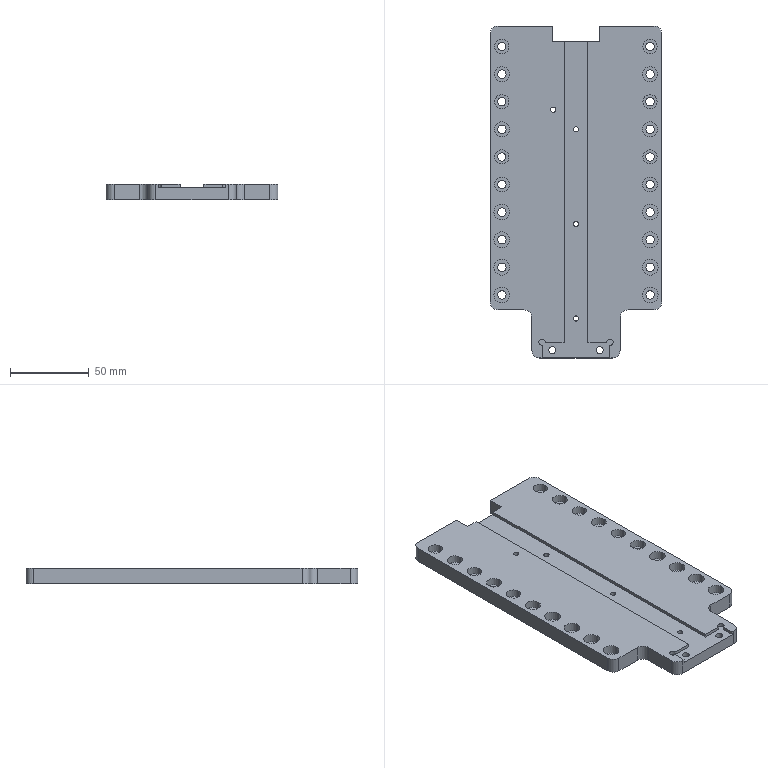Part | SolidWorks | features MoveFace 15, ICE 13, HoleWzd 9, 3DProfileFeature 6, LPattern 6, Fillet 5, Cut 3, Chamfer 2, MirrorPattern 2, Extrusion 1 | 1 solid | 162 faces | box 108.9 x 210.5 x 10 mm | volume 192213 mm3 | cylinder 113 | plane 45 | cone 4 | commonest cylinder face diameters 5.3 x40 10 x24 3.3 x12 9 x12 9.5 x12 8 x6